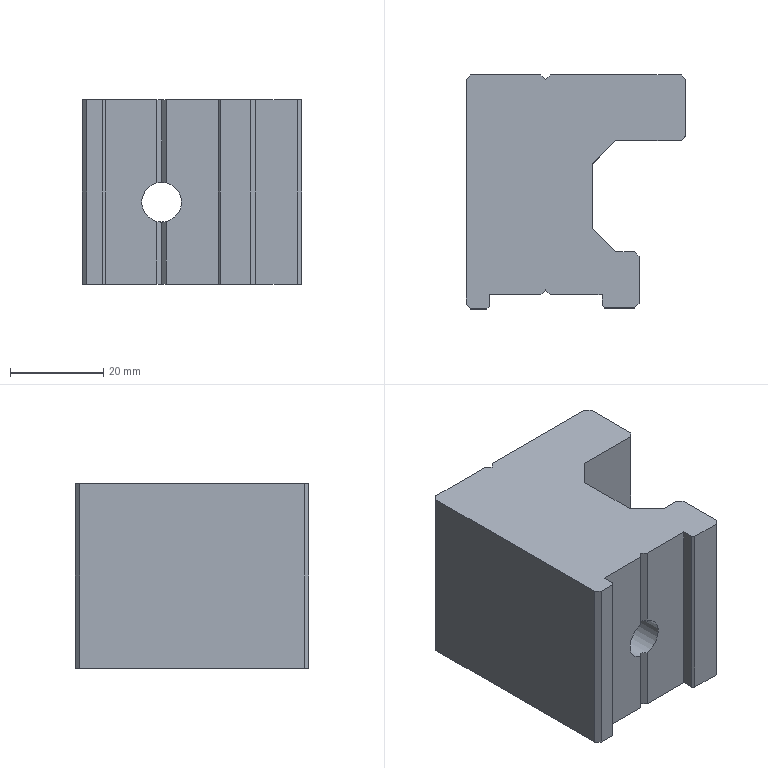Part | NX | features EXTRUDE 3, DATUM_CSYS 2, SKETCH 1 | 1 solid | 37 faces | box 47 x 50 x 39.5 mm | volume 63249 mm3 | plane 35 | cylinder 2 | commonest cylinder face diameters 8.5 x1 14 x1
STEP:
#1=CARTESIAN_POINT('',(5878.887,6899.233,-28.856));
#2=VERTEX_POINT('',#1);
#3=CARTESIAN_POINT('',(5878.887,6899.233,-15.));
#4=VERTEX_POINT('',#3);
#5=CARTESIAN_POINT('',(5879.887,6899.233,-21.928));
#6=DIRECTION('',(0.,1.,0.));
#7=DIRECTION('',(1.,0.,0.));
#8=AXIS2_PLACEMENT_3D('',#5,#6,#7);
#9=CIRCLE('',#8,7.);
#10=EDGE_CURVE('',#2,#4,#9,.T.);
#11=ORIENTED_EDGE('',*,*,#10,.F.);
#12=CARTESIAN_POINT('',(5878.887,6899.233,-39.5));
#13=VERTEX_POINT('',#12);
#14=CARTESIAN_POINT('',(5878.887,6899.233,-39.5));
#15=DIRECTION('',(0.,0.,1.));
#16=VECTOR('',#15,1000.);
#17=LINE('',#14,#16);
#18=EDGE_CURVE('',#13,#2,#17,.T.);
#19=ORIENTED_EDGE('',*,*,#18,.F.);
#20=CARTESIAN_POINT('',(5863.887,6899.233,-39.5));
#21=VERTEX_POINT('',#20);
#22=CARTESIAN_POINT('',(5863.887,6899.233,-39.5));
#23=DIRECTION('',(1.,0.,0.));
#24=VECTOR('',#23,1000.);
#25=LINE('',#22,#24);
#26=EDGE_CURVE('',#21,#13,#25,.T.);
#27=ORIENTED_EDGE('',*,*,#26,.F.);
#28=CARTESIAN_POINT('',(5863.887,6899.233,0.));
#29=VERTEX_POINT('',#28);
#30=CARTESIAN_POINT('',(5863.887,6899.233,-39.5));
#31=DIRECTION('',(0.,0.,1.));
#32=VECTOR('',#31,1000.);
#33=LINE('',#30,#32);
#34=EDGE_CURVE('',#21,#29,#33,.T.);
#35=ORIENTED_EDGE('',*,*,#34,.T.);
#36=CARTESIAN_POINT('',(5878.887,6899.233,0.));
#37=VERTEX_POINT('',#36);
#38=CARTESIAN_POINT('',(5863.887,6899.233,0.));
#39=DIRECTION('',(1.,0.,0.));
#40=VECTOR('',#39,1000.);
#41=LINE('',#38,#40);
#42=EDGE_CURVE('',#29,#37,#41,.T.);
#43=ORIENTED_EDGE('',*,*,#42,.T.);
#44=CARTESIAN_POINT('',(5878.887,6899.233,-39.5));
#45=DIRECTION('',(0.,0.,1.));
#46=VECTOR('',#45,1000.);
#47=LINE('',#44,#46);
#48=EDGE_CURVE('',#4,#37,#47,.T.);
#49=ORIENTED_EDGE('',*,*,#48,.F.);
#50=EDGE_LOOP('',(#11,#19,#27,#35,#43,#49));
#51=FACE_BOUND('',#50,.T.);
#52=CARTESIAN_POINT('',(5863.887,6899.233,-39.5));
#53=DIRECTION('',(0.,-1.,0.));
#54=DIRECTION('',(0.,0.,-1.));
#55=AXIS2_PLACEMENT_3D('',#52,#53,#54);
#56=PLANE('',#55);
#57=ADVANCED_FACE('',(#51),#56,.F.);
#58=CARTESIAN_POINT('',(5880.887,6899.233,-15.));
#59=VERTEX_POINT('',#58);
#60=CARTESIAN_POINT('',(5880.887,6899.233,-28.856));
#61=VERTEX_POINT('',#60);
#62=CARTESIAN_POINT('',(5879.887,6899.233,-21.928));
#63=DIRECTION('',(0.,1.,0.));
#64=DIRECTION('',(1.,0.,0.));
#65=AXIS2_PLACEMENT_3D('',#62,#63,#64);
#66=CIRCLE('',#65,7.);
#67=EDGE_CURVE('',#59,#61,#66,.T.);
#68=ORIENTED_EDGE('',*,*,#67,.F.);
#69=CARTESIAN_POINT('',(5880.887,6899.233,0.));
#70=VERTEX_POINT('',#69);
#71=CARTESIAN_POINT('',(5880.887,6899.233,-39.5));
#72=DIRECTION('',(0.,0.,1.));
#73=VECTOR('',#72,1000.);
#74=LINE('',#71,#73);
#75=EDGE_CURVE('',#59,#70,#74,.T.);
#76=ORIENTED_EDGE('',*,*,#75,.T.);
#77=CARTESIAN_POINT('',(5908.887,6899.233,0.));
#78=VERTEX_POINT('',#77);
#79=CARTESIAN_POINT('',(5880.887,6899.233,0.));
#80=DIRECTION('',(1.,0.,0.));
#81=VECTOR('',#80,1000.);
#82=LINE('',#79,#81);
#83=EDGE_CURVE('',#70,#78,#82,.T.);
#84=ORIENTED_EDGE('',*,*,#83,.T.);
#85=CARTESIAN_POINT('',(5908.887,6899.233,-39.5));
#86=VERTEX_POINT('',#85);
#87=CARTESIAN_POINT('',(5908.887,6899.233,-39.5));
#88=DIRECTION('',(0.,0.,1.));
#89=VECTOR('',#88,1000.);
#90=LINE('',#87,#89);
#91=EDGE_CURVE('',#86,#78,#90,.T.);
#92=ORIENTED_EDGE('',*,*,#91,.F.);
#93=CARTESIAN_POINT('',(5880.887,6899.233,-39.5));
#94=VERTEX_POINT('',#93);
#95=CARTESIAN_POINT('',(5880.887,6899.233,-39.5));
#96=DIRECTION('',(1.,0.,0.));
#97=VECTOR('',#96,1000.);
#98=LINE('',#95,#97);
#99=EDGE_CURVE('',#94,#86,#98,.T.);
#100=ORIENTED_EDGE('',*,*,#99,.F.);
#101=CARTESIAN_POINT('',(5880.887,6899.233,-39.5));
#102=DIRECTION('',(0.,0.,1.));
#103=VECTOR('',#102,1000.);
#104=LINE('',#101,#103);
#105=EDGE_CURVE('',#94,#61,#104,.T.);
#106=ORIENTED_EDGE('',*,*,#105,.T.);
#107=EDGE_LOOP('',(#68,#76,#84,#92,#100,#106));
#108=FACE_BOUND('',#107,.T.);
#109=CARTESIAN_POINT('',(5880.887,6899.233,-39.5));
#110=DIRECTION('',(0.,-1.,0.));
#111=DIRECTION('',(0.,0.,-1.));
#112=AXIS2_PLACEMENT_3D('',#109,#110,#111);
#113=PLANE('',#112);
#114=ADVANCED_FACE('',(#108),#113,.F.);
#115=CARTESIAN_POINT('',(5878.887,6852.233,-17.797));
#116=VERTEX_POINT('',#115);
#117=CARTESIAN_POINT('',(5878.887,6852.233,-26.059));
#118=VERTEX_POINT('',#117);
#119=CARTESIAN_POINT('',(5879.887,6852.233,-21.928));
#120=DIRECTION('',(0.,1.,0.));
#121=DIRECTION('',(0.,0.,1.));
#122=AXIS2_PLACEMENT_3D('',#119,#120,#121);
#123=CIRCLE('',#122,4.25);
#124=EDGE_CURVE('',#116,#118,#123,.F.);
#125=ORIENTED_EDGE('',*,*,#124,.T.);
#126=CARTESIAN_POINT('',(5879.887,6853.233,-26.178));
#127=VERTEX_POINT('',#126);
#128=CARTESIAN_POINT('',(5879.887,6853.233,-21.928));
#129=DIRECTION('',(-0.7071,0.7071,0.));
#130=DIRECTION('',(0.7071,0.7071,0.));
#131=AXIS2_PLACEMENT_3D('',#128,#129,#130);
#132=ELLIPSE('',#131,6.01,4.25);
#133=EDGE_CURVE('',#118,#127,#132,.F.);
#134=ORIENTED_EDGE('',*,*,#133,.T.);
#135=CARTESIAN_POINT('',(5880.887,6852.233,-26.059));
#136=VERTEX_POINT('',#135);
#137=CARTESIAN_POINT('',(5879.887,6853.233,-21.928));
#138=DIRECTION('',(0.7071,0.7071,0.));
#139=DIRECTION('',(-0.7071,0.7071,0.));
#140=AXIS2_PLACEMENT_3D('',#137,#138,#139);
#141=ELLIPSE('',#140,6.01,4.25);
#142=EDGE_CURVE('',#127,#136,#141,.F.);
#143=ORIENTED_EDGE('',*,*,#142,.T.);
#144=CARTESIAN_POINT('',(5880.887,6852.233,-17.797));
#145=VERTEX_POINT('',#144);
#146=CARTESIAN_POINT('',(5879.887,6852.233,-21.928));
#147=DIRECTION('',(0.,1.,0.));
#148=DIRECTION('',(0.,0.,1.));
#149=AXIS2_PLACEMENT_3D('',#146,#147,#148);
#150=CIRCLE('',#149,4.25);
#151=EDGE_CURVE('',#136,#145,#150,.F.);
#152=ORIENTED_EDGE('',*,*,#151,.T.);
#153=CARTESIAN_POINT('',(5879.887,6853.233,-17.678));
#154=VERTEX_POINT('',#153);
#155=CARTESIAN_POINT('',(5879.887,6853.233,-21.928));
#156=DIRECTION('',(0.7071,0.7071,0.));
#157=DIRECTION('',(-0.7071,0.7071,0.));
#158=AXIS2_PLACEMENT_3D('',#155,#156,#157);
#159=ELLIPSE('',#158,6.01,4.25);
#160=EDGE_CURVE('',#145,#154,#159,.F.);
#161=ORIENTED_EDGE('',*,*,#160,.T.);
#162=CARTESIAN_POINT('',(5879.887,6853.233,-21.928));
#163=DIRECTION('',(-0.7071,0.7071,0.));
#164=DIRECTION('',(0.7071,0.7071,0.));
#165=AXIS2_PLACEMENT_3D('',#162,#163,#164);
#166=ELLIPSE('',#165,6.01,4.25);
#167=EDGE_CURVE('',#154,#116,#166,.F.);
#168=ORIENTED_EDGE('',*,*,#167,.T.);
#169=EDGE_LOOP('',(#125,#134,#143,#152,#161,#168));
#170=FACE_BOUND('',#169,.T.);
#171=CARTESIAN_POINT('',(5879.887,6887.233,-17.678));
#172=VERTEX_POINT('',#171);
#173=CARTESIAN_POINT('',(5879.887,6887.233,-21.928));
#174=DIRECTION('',(0.,1.,0.));
#175=DIRECTION('',(0.,0.,1.));
#176=AXIS2_PLACEMENT_3D('',#173,#174,#175);
#177=CIRCLE('',#176,4.25);
#178=EDGE_CURVE('',#172,#172,#177,.F.);
#179=ORIENTED_EDGE('',*,*,#178,.F.);
#180=EDGE_LOOP('',(#179));
#181=FACE_BOUND('',#180,.T.);
#182=CARTESIAN_POINT('',(5879.887,-48100.767,-21.928));
#183=DIRECTION('',(0.,1.,0.));
#184=DIRECTION('',(0.,0.,1.));
#185=AXIS2_PLACEMENT_3D('',#182,#183,#184);
#186=CYLINDRICAL_SURFACE('',#185,4.25);
#187=ADVANCED_FACE('',(#170,#181),#186,.F.);
#188=ORIENTED_EDGE('',*,*,#18,.T.);
#189=CARTESIAN_POINT('',(5879.887,6898.233,-28.928));
#190=VERTEX_POINT('',#189);
#191=CARTESIAN_POINT('',(5879.887,6898.233,-21.928));
#192=DIRECTION('',(-0.7071,-0.7071,0.));
#193=DIRECTION('',(-0.7071,0.7071,0.));
#194=AXIS2_PLACEMENT_3D('',#191,#192,#193);
#195=ELLIPSE('',#194,9.899,7.);
#196=EDGE_CURVE('',#2,#190,#195,.T.);
#197=ORIENTED_EDGE('',*,*,#196,.T.);
#198=CARTESIAN_POINT('',(5879.887,6898.233,-39.5));
#199=VERTEX_POINT('',#198);
#200=CARTESIAN_POINT('',(5879.887,6898.233,-39.5));
#201=DIRECTION('',(0.,0.,1.));
#202=VECTOR('',#201,1000.);
#203=LINE('',#200,#202);
#204=EDGE_CURVE('',#199,#190,#203,.T.);
#205=ORIENTED_EDGE('',*,*,#204,.F.);
#206=CARTESIAN_POINT('',(5878.887,6899.233,-39.5));
#207=DIRECTION('',(0.7071,-0.7071,0.));
#208=VECTOR('',#207,1000.);
#209=LINE('',#206,#208);
#210=EDGE_CURVE('',#13,#199,#209,.T.);
#211=ORIENTED_EDGE('',*,*,#210,.F.);
#212=EDGE_LOOP('',(#188,#197,#205,#211));
#213=FACE_BOUND('',#212,.T.);
#214=CARTESIAN_POINT('',(5878.887,6899.233,-39.5));
#215=DIRECTION('',(-0.7071,-0.7071,0.));
#216=DIRECTION('',(0.7071,-0.7071,0.));
#217=AXIS2_PLACEMENT_3D('',#214,#215,#216);
#218=PLANE('',#217);
#219=ADVANCED_FACE('',(#213),#218,.F.);
#220=ORIENTED_EDGE('',*,*,#75,.F.);
#221=CARTESIAN_POINT('',(5879.887,6898.233,-14.928));
#222=VERTEX_POINT('',#221);
#223=CARTESIAN_POINT('',(5879.887,6898.233,-21.928));
#224=DIRECTION('',(0.7071,-0.7071,0.));
#225=DIRECTION('',(0.7071,0.7071,0.));
#226=AXIS2_PLACEMENT_3D('',#223,#224,#225);
#227=ELLIPSE('',#226,9.899,7.);
#228=EDGE_CURVE('',#59,#222,#227,.T.);
#229=ORIENTED_EDGE('',*,*,#228,.T.);
#230=CARTESIAN_POINT('',(5879.887,6898.233,0.));
#231=VERTEX_POINT('',#230);
#232=CARTESIAN_POINT('',(5879.887,6898.233,-39.5));
#233=DIRECTION('',(0.,0.,1.));
#234=VECTOR('',#233,1000.);
#235=LINE('',#232,#234);
#236=EDGE_CURVE('',#222,#231,#235,.T.);
#237=ORIENTED_EDGE('',*,*,#236,.T.);
#238=CARTESIAN_POINT('',(5879.887,6898.233,0.));
#239=DIRECTION('',(0.7071,0.7071,0.));
#240=VECTOR('',#239,1000.);
#241=LINE('',#238,#240);
#242=EDGE_CURVE('',#231,#70,#241,.T.);
#243=ORIENTED_EDGE('',*,*,#242,.T.);
#244=EDGE_LOOP('',(#220,#229,#237,#243));
#245=FACE_BOUND('',#244,.T.);
#246=CARTESIAN_POINT('',(5879.887,6898.233,-39.5));
#247=DIRECTION('',(0.7071,-0.7071,0.));
#248=DIRECTION('',(0.7071,0.7071,0.));
#249=AXIS2_PLACEMENT_3D('',#246,#247,#248);
#250=PLANE('',#249);
#251=ADVANCED_FACE('',(#245),#250,.F.);
#252=ORIENTED_EDGE('',*,*,#151,.F.);
#253=CARTESIAN_POINT('',(5880.887,6852.233,-39.5));
#254=VERTEX_POINT('',#253);
#255=CARTESIAN_POINT('',(5880.887,6852.233,-39.5));
#256=DIRECTION('',(0.,0.,1.));
#257=VECTOR('',#256,1000.);
#258=LINE('',#255,#257);
#259=EDGE_CURVE('',#254,#136,#258,.T.);
#260=ORIENTED_EDGE('',*,*,#259,.F.);
#261=CARTESIAN_POINT('',(5891.962,6852.233,-39.5));
#262=VERTEX_POINT('',#261);
#263=CARTESIAN_POINT('',(5891.962,6852.233,-39.5));
#264=DIRECTION('',(-1.,0.,0.));
#265=VECTOR('',#264,1000.);
#266=LINE('',#263,#265);
#267=EDGE_CURVE('',#262,#254,#266,.T.);
#268=ORIENTED_EDGE('',*,*,#267,.F.);
#269=CARTESIAN_POINT('',(5891.962,6852.233,0.));
#270=VERTEX_POINT('',#269);
#271=CARTESIAN_POINT('',(5891.962,6852.233,-39.5));
#272=DIRECTION('',(0.,0.,1.));
#273=VECTOR('',#272,1000.);
#274=LINE('',#271,#273);
#275=EDGE_CURVE('',#262,#270,#274,.T.);
#276=ORIENTED_EDGE('',*,*,#275,.T.);
#277=CARTESIAN_POINT('',(5880.887,6852.233,0.));
#278=VERTEX_POINT('',#277);
#279=CARTESIAN_POINT('',(5891.962,6852.233,0.));
#280=DIRECTION('',(-1.,0.,0.));
#281=VECTOR('',#280,1000.);
#282=LINE('',#279,#281);
#283=EDGE_CURVE('',#270,#278,#282,.T.);
#284=ORIENTED_EDGE('',*,*,#283,.T.);
#285=CARTESIAN_POINT('',(5880.887,6852.233,-39.5));
#286=DIRECTION('',(0.,0.,1.));
#287=VECTOR('',#286,1000.);
#288=LINE('',#285,#287);
#289=EDGE_CURVE('',#145,#278,#288,.T.);
#290=ORIENTED_EDGE('',*,*,#289,.F.);
#291=EDGE_LOOP('',(#252,#260,#268,#276,#284,#290));
#292=FACE_BOUND('',#291,.T.);
#293=CARTESIAN_POINT('',(5891.962,6852.233,-39.5));
#294=DIRECTION('',(0.,1.,0.));
#295=DIRECTION('',(0.,0.,1.));
#296=AXIS2_PLACEMENT_3D('',#293,#294,#295);
#297=PLANE('',#296);
#298=ADVANCED_FACE('',(#292),#297,.F.);
#299=ORIENTED_EDGE('',*,*,#142,.F.);
#300=CARTESIAN_POINT('',(5879.887,6853.233,-39.5));
#301=VERTEX_POINT('',#300);
#302=CARTESIAN_POINT('',(5879.887,6853.233,-39.5));
#303=DIRECTION('',(0.,0.,1.));
#304=VECTOR('',#303,1000.);
#305=LINE('',#302,#304);
#306=EDGE_CURVE('',#301,#127,#305,.T.);
#307=ORIENTED_EDGE('',*,*,#306,.F.);
#308=CARTESIAN_POINT('',(5880.887,6852.233,-39.5));
#309=DIRECTION('',(-0.7071,0.7071,0.));
#310=VECTOR('',#309,1000.);
#311=LINE('',#308,#310);
#312=EDGE_CURVE('',#254,#301,#311,.T.);
#313=ORIENTED_EDGE('',*,*,#312,.F.);
#314=ORIENTED_EDGE('',*,*,#259,.T.);
#315=EDGE_LOOP('',(#299,#307,#313,#314));
#316=FACE_BOUND('',#315,.T.);
#317=CARTESIAN_POINT('',(5880.887,6852.233,-39.5));
#318=DIRECTION('',(0.7071,0.7071,0.));
#319=DIRECTION('',(-0.7071,0.7071,0.));
#320=AXIS2_PLACEMENT_3D('',#317,#318,#319);
#321=PLANE('',#320);
#322=ADVANCED_FACE('',(#316),#321,.F.);
#323=ORIENTED_EDGE('',*,*,#160,.F.);
#324=ORIENTED_EDGE('',*,*,#289,.T.);
#325=CARTESIAN_POINT('',(5879.887,6853.233,0.));
#326=VERTEX_POINT('',#325);
#327=CARTESIAN_POINT('',(5880.887,6852.233,0.));
#328=DIRECTION('',(-0.7071,0.7071,0.));
#329=VECTOR('',#328,1000.);
#330=LINE('',#327,#329);
#331=EDGE_CURVE('',#278,#326,#330,.T.);
#332=ORIENTED_EDGE('',*,*,#331,.T.);
#333=CARTESIAN_POINT('',(5879.887,6853.233,-39.5));
#334=DIRECTION('',(0.,0.,1.));
#335=VECTOR('',#334,1000.);
#336=LINE('',#333,#335);
#337=EDGE_CURVE('',#154,#326,#336,.T.);
#338=ORIENTED_EDGE('',*,*,#337,.F.);
#339=EDGE_LOOP('',(#323,#324,#332,#338));
#340=FACE_BOUND('',#339,.T.);
#341=CARTESIAN_POINT('',(5880.887,6852.233,-39.5));
#342=DIRECTION('',(0.7071,0.7071,0.));
#343=DIRECTION('',(-0.7071,0.7071,0.));
#344=AXIS2_PLACEMENT_3D('',#341,#342,#343);
#345=PLANE('',#344);
#346=ADVANCED_FACE('',(#340),#345,.F.);
#347=ORIENTED_EDGE('',*,*,#167,.F.);
#348=ORIENTED_EDGE('',*,*,#337,.T.);
#349=CARTESIAN_POINT('',(5878.887,6852.233,0.));
#350=VERTEX_POINT('',#349);
#351=CARTESIAN_POINT('',(5879.887,6853.233,0.));
#352=DIRECTION('',(-0.7071,-0.7071,0.));
#353=VECTOR('',#352,1000.);
#354=LINE('',#351,#353);
#355=EDGE_CURVE('',#326,#350,#354,.T.);
#356=ORIENTED_EDGE('',*,*,#355,.T.);
#357=CARTESIAN_POINT('',(5878.887,6852.233,-39.5));
#358=DIRECTION('',(0.,0.,1.));
#359=VECTOR('',#358,1000.);
#360=LINE('',#357,#359);
#361=EDGE_CURVE('',#116,#350,#360,.T.);
#362=ORIENTED_EDGE('',*,*,#361,.F.);
#363=EDGE_LOOP('',(#347,#348,#356,#362));
#364=FACE_BOUND('',#363,.T.);
#365=CARTESIAN_POINT('',(5879.887,6853.233,-39.5));
#366=DIRECTION('',(-0.7071,0.7071,0.));
#367=DIRECTION('',(-0.7071,-0.7071,0.));
#368=AXIS2_PLACEMENT_3D('',#365,#366,#367);
#369=PLANE('',#368);
#370=ADVANCED_FACE('',(#364),#369,.F.);
#371=ORIENTED_EDGE('',*,*,#133,.F.);
#372=CARTESIAN_POINT('',(5878.887,6852.233,-39.5));
#373=VERTEX_POINT('',#372);
#374=CARTESIAN_POINT('',(5878.887,6852.233,-39.5));
#375=DIRECTION('',(0.,0.,1.));
#376=VECTOR('',#375,1000.);
#377=LINE('',#374,#376);
#378=EDGE_CURVE('',#373,#118,#377,.T.);
#379=ORIENTED_EDGE('',*,*,#378,.F.);
#380=CARTESIAN_POINT('',(5879.887,6853.233,-39.5));
#381=DIRECTION('',(-0.7071,-0.7071,0.));
#382=VECTOR('',#381,1000.);
#383=LINE('',#380,#382);
#384=EDGE_CURVE('',#301,#373,#383,.T.);
#385=ORIENTED_EDGE('',*,*,#384,.F.);
#386=ORIENTED_EDGE('',*,*,#306,.T.);
#387=EDGE_LOOP('',(#371,#379,#385,#386));
#388=FACE_BOUND('',#387,.T.);
#389=CARTESIAN_POINT('',(5879.887,6853.233,-39.5));
#390=DIRECTION('',(-0.7071,0.7071,0.));
#391=DIRECTION('',(-0.7071,-0.7071,0.));
#392=AXIS2_PLACEMENT_3D('',#389,#390,#391);
#393=PLANE('',#392);
#394=ADVANCED_FACE('',(#388),#393,.F.);
#395=ORIENTED_EDGE('',*,*,#124,.F.);
#396=ORIENTED_EDGE('',*,*,#361,.T.);
#397=CARTESIAN_POINT('',(5867.812,6852.233,0.));
#398=VERTEX_POINT('',#397);
#399=CARTESIAN_POINT('',(5878.887,6852.233,0.));
#400=DIRECTION('',(-1.,0.,0.));
#401=VECTOR('',#400,1000.);
#402=LINE('',#399,#401);
#403=EDGE_CURVE('',#350,#398,#402,.T.);
#404=ORIENTED_EDGE('',*,*,#403,.T.);
#405=CARTESIAN_POINT('',(5867.812,6852.233,-39.5));
#406=VERTEX_POINT('',#405);
#407=CARTESIAN_POINT('',(5867.812,6852.233,-39.5));
#408=DIRECTION('',(0.,0.,1.));
#409=VECTOR('',#408,1000.);
#410=LINE('',#407,#409);
#411=EDGE_CURVE('',#406,#398,#410,.T.);
#412=ORIENTED_EDGE('',*,*,#411,.F.);
#413=CARTESIAN_POINT('',(5878.887,6852.233,-39.5));
#414=DIRECTION('',(-1.,0.,0.));
#415=VECTOR('',#414,1000.);
#416=LINE('',#413,#415);
#417=EDGE_CURVE('',#373,#406,#416,.T.);
#418=ORIENTED_EDGE('',*,*,#417,.F.);
#419=ORIENTED_EDGE('',*,*,#378,.T.);
#420=EDGE_LOOP('',(#395,#396,#404,#412,#418,#419));
#421=FACE_BOUND('',#420,.T.);
#422=CARTESIAN_POINT('',(5878.887,6852.233,-39.5));
#423=DIRECTION('',(0.,1.,0.));
#424=DIRECTION('',(0.,0.,1.));
#425=AXIS2_PLACEMENT_3D('',#422,#423,#424);
#426=PLANE('',#425);
#427=ADVANCED_FACE('',(#421),#426,.F.);
#428=CARTESIAN_POINT('',(5862.887,6850.233,0.));
#429=VERTEX_POINT('',#428);
#430=CARTESIAN_POINT('',(5862.887,6898.233,0.));
#431=VERTEX_POINT('',#430);
#432=CARTESIAN_POINT('',(5862.887,6850.233,0.));
#433=DIRECTION('',(0.,1.,0.));
#434=VECTOR('',#433,1000.);
#435=LINE('',#432,#434);
#436=EDGE_CURVE('',#429,#431,#435,.T.);
#437=ORIENTED_EDGE('',*,*,#436,.T.);
#438=CARTESIAN_POINT('',(5862.887,6898.233,-39.5));
#439=VERTEX_POINT('',#438);
#440=CARTESIAN_POINT('',(5862.887,6898.233,-39.5));
#441=DIRECTION('',(0.,0.,1.));
#442=VECTOR('',#441,1000.);
#443=LINE('',#440,#442);
#444=EDGE_CURVE('',#439,#431,#443,.T.);
#445=ORIENTED_EDGE('',*,*,#444,.F.);
#446=CARTESIAN_POINT('',(5862.887,6850.233,-39.5));
#447=VERTEX_POINT('',#446);
#448=CARTESIAN_POINT('',(5862.887,6850.233,-39.5));
#449=DIRECTION('',(0.,1.,0.));
#450=VECTOR('',#449,1000.);
#451=LINE('',#448,#450);
#452=EDGE_CURVE('',#447,#439,#451,.T.);
#453=ORIENTED_EDGE('',*,*,#452,.F.);
#454=CARTESIAN_POINT('',(5862.887,6850.233,-39.5));
#455=DIRECTION('',(0.,0.,1.));
#456=VECTOR('',#455,1000.);
#457=LINE('',#454,#456);
#458=EDGE_CURVE('',#447,#429,#457,.T.);
#459=ORIENTED_EDGE('',*,*,#458,.T.);
#460=EDGE_LOOP('',(#437,#445,#453,#459));
#461=FACE_BOUND('',#460,.T.);
#462=CARTESIAN_POINT('',(5862.887,6850.233,-39.5));
#463=DIRECTION('',(1.,0.,0.));
#464=DIRECTION('',(0.,0.,-1.));
#465=AXIS2_PLACEMENT_3D('',#462,#463,#464);
#466=PLANE('',#465);
#467=ADVANCED_FACE('',(#461),#466,.F.);
#468=CARTESIAN_POINT('',(5862.887,6898.233,0.));
#469=DIRECTION('',(0.7071,0.7071,0.));
#470=VECTOR('',#469,1000.);
#471=LINE('',#468,#470);
#472=EDGE_CURVE('',#431,#29,#471,.T.);
#473=ORIENTED_EDGE('',*,*,#472,.T.);
#474=ORIENTED_EDGE('',*,*,#34,.F.);
#475=CARTESIAN_POINT('',(5862.887,6898.233,-39.5));
#476=DIRECTION('',(0.7071,0.7071,0.));
#477=VECTOR('',#476,1000.);
#478=LINE('',#475,#477);
#479=EDGE_CURVE('',#439,#21,#478,.T.);
#480=ORIENTED_EDGE('',*,*,#479,.F.);
#481=ORIENTED_EDGE('',*,*,#444,.T.);
#482=EDGE_LOOP('',(#473,#474,#480,#481));
#483=FACE_BOUND('',#482,.T.);
#484=CARTESIAN_POINT('',(5862.887,6898.233,-39.5));
#485=DIRECTION('',(0.7071,-0.7071,0.));
#486=DIRECTION('',(0.7071,0.7071,0.));
#487=AXIS2_PLACEMENT_3D('',#484,#485,#486);
#488=PLANE('',#487);
#489=ADVANCED_FACE('',(#483),#488,.F.);
#490=ORIENTED_EDGE('',*,*,#236,.F.);
#491=CARTESIAN_POINT('',(5879.887,6898.233,-21.928));
#492=DIRECTION('',(-0.7071,-0.7071,0.));
#493=DIRECTION('',(-0.7071,0.7071,0.));
#494=AXIS2_PLACEMENT_3D('',#491,#492,#493);
#495=ELLIPSE('',#494,9.899,7.);
#496=EDGE_CURVE('',#222,#4,#495,.T.);
#497=ORIENTED_EDGE('',*,*,#496,.T.);
#498=ORIENTED_EDGE('',*,*,#48,.T.);
#499=CARTESIAN_POINT('',(5878.887,6899.233,0.));
#500=DIRECTION('',(0.7071,-0.7071,0.));
#501=VECTOR('',#500,1000.);
#502=LINE('',#499,#501);
#503=EDGE_CURVE('',#37,#231,#502,.T.);
#504=ORIENTED_EDGE('',*,*,#503,.T.);
#505=EDGE_LOOP('',(#490,#497,#498,#504));
#506=FACE_BOUND('',#505,.T.);
#507=CARTESIAN_POINT('',(5878.887,6899.233,-39.5));
#508=DIRECTION('',(-0.7071,-0.7071,0.));
#509=DIRECTION('',(0.7071,-0.7071,0.));
#510=AXIS2_PLACEMENT_3D('',#507,#508,#509);
#511=PLANE('',#510);
#512=ADVANCED_FACE('',(#506),#511,.F.);
#513=ORIENTED_EDGE('',*,*,#204,.T.);
#514=CARTESIAN_POINT('',(5879.887,6898.233,-21.928));
#515=DIRECTION('',(0.7071,-0.7071,0.));
#516=DIRECTION('',(0.7071,0.7071,0.));
#517=AXIS2_PLACEMENT_3D('',#514,#515,#516);
#518=ELLIPSE('',#517,9.899,7.);
#519=EDGE_CURVE('',#190,#61,#518,.T.);
#520=ORIENTED_EDGE('',*,*,#519,.T.);
#521=ORIENTED_EDGE('',*,*,#105,.F.);
#522=CARTESIAN_POINT('',(5879.887,6898.233,-39.5));
#523=DIRECTION('',(0.7071,0.7071,0.));
#524=VECTOR('',#523,1000.);
#525=LINE('',#522,#524);
#526=EDGE_CURVE('',#199,#94,#525,.T.);
#527=ORIENTED_EDGE('',*,*,#526,.F.);
#528=EDGE_LOOP('',(#513,#520,#521,#527));
#529=FACE_BOUND('',#528,.T.);
#530=CARTESIAN_POINT('',(5879.887,6898.233,-39.5));
#531=DIRECTION('',(0.7071,-0.7071,0.));
#532=DIRECTION('',(0.7071,0.7071,0.));
#533=AXIS2_PLACEMENT_3D('',#530,#531,#532);
#534=PLANE('',#533);
#535=ADVANCED_FACE('',(#529),#534,.F.);
#536=CARTESIAN_POINT('',(5909.887,6898.233,0.));
#537=VERTEX_POINT('',#536);
#538=CARTESIAN_POINT('',(5908.887,6899.233,0.));
#539=DIRECTION('',(0.7071,-0.7071,0.));
#540=VECTOR('',#539,1000.);
#541=LINE('',#538,#540);
#542=EDGE_CURVE('',#78,#537,#541,.T.);
#543=ORIENTED_EDGE('',*,*,#542,.T.);
#544=CARTESIAN_POINT('',(5909.887,6898.233,-39.5));
#545=VERTEX_POINT('',#544);
#546=CARTESIAN_POINT('',(5909.887,6898.233,-39.5));
#547=DIRECTION('',(0.,0.,1.));
#548=VECTOR('',#547,1000.);
#549=LINE('',#546,#548);
#550=EDGE_CURVE('',#545,#537,#549,.T.);
#551=ORIENTED_EDGE('',*,*,#550,.F.);
#552=CARTESIAN_POINT('',(5908.887,6899.233,-39.5));
#553=DIRECTION('',(0.7071,-0.7071,0.));
#554=VECTOR('',#553,1000.);
#555=LINE('',#552,#554);
#556=EDGE_CURVE('',#86,#545,#555,.T.);
#557=ORIENTED_EDGE('',*,*,#556,.F.);
#558=ORIENTED_EDGE('',*,*,#91,.T.);
#559=EDGE_LOOP('',(#543,#551,#557,#558));
#560=FACE_BOUND('',#559,.T.);
#561=CARTESIAN_POINT('',(5908.887,6899.233,-39.5));
#562=DIRECTION('',(-0.7071,-0.7071,0.));
#563=DIRECTION('',(0.7071,-0.7071,0.));
#564=AXIS2_PLACEMENT_3D('',#561,#562,#563);
#565=PLANE('',#564);
#566=ADVANCED_FACE('',(#560),#565,.F.);
#567=CARTESIAN_POINT('',(5909.887,6886.233,0.));
#568=VERTEX_POINT('',#567);
#569=CARTESIAN_POINT('',(5909.887,6898.233,0.));
#570=DIRECTION('',(0.,-1.,0.));
#571=VECTOR('',#570,1000.);
#572=LINE('',#569,#571);
#573=EDGE_CURVE('',#537,#568,#572,.T.);
#574=ORIENTED_EDGE('',*,*,#573,.T.);
#575=CARTESIAN_POINT('',(5909.887,6886.233,-39.5));
#576=VERTEX_POINT('',#575);
#577=CARTESIAN_POINT('',(5909.887,6886.233,-39.5));
#578=DIRECTION('',(0.,0.,1.));
#579=VECTOR('',#578,1000.);
#580=LINE('',#577,#579);
#581=EDGE_CURVE('',#576,#568,#580,.T.);
#582=ORIENTED_EDGE('',*,*,#581,.F.);
#583=CARTESIAN_POINT('',(5909.887,6898.233,-39.5));
#584=DIRECTION('',(0.,-1.,0.));
#585=VECTOR('',#584,1000.);
#586=LINE('',#583,#585);
#587=EDGE_CURVE('',#545,#576,#586,.T.);
#588=ORIENTED_EDGE('',*,*,#587,.F.);
#589=ORIENTED_EDGE('',*,*,#550,.T.);
#590=EDGE_LOOP('',(#574,#582,#588,#589));
#591=FACE_BOUND('',#590,.T.);
#592=CARTESIAN_POINT('',(5909.887,6898.233,-39.5));
#593=DIRECTION('',(-1.,0.,0.));
#594=DIRECTION('',(0.,0.,1.));
#595=AXIS2_PLACEMENT_3D('',#592,#593,#594);
#596=PLANE('',#595);
#597=ADVANCED_FACE('',(#591),#596,.F.);
#598=CARTESIAN_POINT('',(5908.887,6885.233,0.));
#599=VERTEX_POINT('',#598);
#600=CARTESIAN_POINT('',(5909.887,6886.233,0.));
#601=DIRECTION('',(-0.7071,-0.7071,0.));
#602=VECTOR('',#601,1000.);
#603=LINE('',#600,#602);
#604=EDGE_CURVE('',#568,#599,#603,.T.);
#605=ORIENTED_EDGE('',*,*,#604,.T.);
#606=CARTESIAN_POINT('',(5908.887,6885.233,-39.5));
#607=VERTEX_POINT('',#606);
#608=CARTESIAN_POINT('',(5908.887,6885.233,-39.5));
#609=DIRECTION('',(0.,0.,1.));
#610=VECTOR('',#609,1000.);
#611=LINE('',#608,#610);
#612=EDGE_CURVE('',#607,#599,#611,.T.);
#613=ORIENTED_EDGE('',*,*,#612,.F.);
#614=CARTESIAN_POINT('',(5909.887,6886.233,-39.5));
#615=DIRECTION('',(-0.7071,-0.7071,0.));
#616=VECTOR('',#615,1000.);
#617=LINE('',#614,#616);
#618=EDGE_CURVE('',#576,#607,#617,.T.);
#619=ORIENTED_EDGE('',*,*,#618,.F.);
#620=ORIENTED_EDGE('',*,*,#581,.T.);
#621=EDGE_LOOP('',(#605,#613,#619,#620));
#622=FACE_BOUND('',#621,.T.);
#623=CARTESIAN_POINT('',(5909.887,6886.233,-39.5));
#624=DIRECTION('',(-0.7071,0.7071,0.));
#625=DIRECTION('',(-0.7071,-0.7071,0.));
#626=AXIS2_PLACEMENT_3D('',#623,#624,#625);
#627=PLANE('',#626);
#628=ADVANCED_FACE('',(#622),#627,.F.);
#629=CARTESIAN_POINT('',(5894.887,6885.233,0.));
#630=VERTEX_POINT('',#629);
#631=CARTESIAN_POINT('',(5908.887,6885.233,0.));
#632=DIRECTION('',(-1.,0.,0.));
#633=VECTOR('',#632,1000.);
#634=LINE('',#631,#633);
#635=EDGE_CURVE('',#599,#630,#634,.T.);
#636=ORIENTED_EDGE('',*,*,#635,.T.);
#637=CARTESIAN_POINT('',(5894.887,6885.233,-39.5));
#638=VERTEX_POINT('',#637);
#639=CARTESIAN_POINT('',(5894.887,6885.233,-39.5));
#640=DIRECTION('',(0.,0.,1.));
#641=VECTOR('',#640,1000.);
#642=LINE('',#639,#641);
#643=EDGE_CURVE('',#638,#630,#642,.T.);
#644=ORIENTED_EDGE('',*,*,#643,.F.);
#645=CARTESIAN_POINT('',(5908.887,6885.233,-39.5));
#646=DIRECTION('',(-1.,0.,0.));
#647=VECTOR('',#646,1000.);
#648=LINE('',#645,#647);
#649=EDGE_CURVE('',#607,#638,#648,.T.);
#650=ORIENTED_EDGE('',*,*,#649,.F.);
#651=ORIENTED_EDGE('',*,*,#612,.T.);
#652=EDGE_LOOP('',(#636,#644,#650,#651));
#653=FACE_BOUND('',#652,.T.);
#654=CARTESIAN_POINT('',(5908.887,6885.233,-39.5));
#655=DIRECTION('',(0.,1.,0.));
#656=DIRECTION('',(0.,0.,1.));
#657=AXIS2_PLACEMENT_3D('',#654,#655,#656);
#658=PLANE('',#657);
#659=ADVANCED_FACE('',(#653),#658,.F.);
#660=CARTESIAN_POINT('',(5889.887,6880.233,0.));
#661=VERTEX_POINT('',#660);
#662=CARTESIAN_POINT('',(5894.887,6885.233,0.));
#663=DIRECTION('',(-0.7071,-0.7071,0.));
#664=VECTOR('',#663,1000.);
#665=LINE('',#662,#664);
#666=EDGE_CURVE('',#630,#661,#665,.T.);
#667=ORIENTED_EDGE('',*,*,#666,.T.);
#668=CARTESIAN_POINT('',(5889.887,6880.233,-39.5));
#669=VERTEX_POINT('',#668);
#670=CARTESIAN_POINT('',(5889.887,6880.233,-39.5));
#671=DIRECTION('',(0.,0.,1.));
#672=VECTOR('',#671,1000.);
#673=LINE('',#670,#672);
#674=EDGE_CURVE('',#669,#661,#673,.T.);
#675=ORIENTED_EDGE('',*,*,#674,.F.);
#676=CARTESIAN_POINT('',(5894.887,6885.233,-39.5));
#677=DIRECTION('',(-0.7071,-0.7071,0.));
#678=VECTOR('',#677,1000.);
#679=LINE('',#676,#678);
#680=EDGE_CURVE('',#638,#669,#679,.T.);
#681=ORIENTED_EDGE('',*,*,#680,.F.);
#682=ORIENTED_EDGE('',*,*,#643,.T.);
#683=EDGE_LOOP('',(#667,#675,#681,#682));
#684=FACE_BOUND('',#683,.T.);
#685=CARTESIAN_POINT('',(5894.887,6885.233,-39.5));
#686=DIRECTION('',(-0.7071,0.7071,0.));
#687=DIRECTION('',(-0.7071,-0.7071,0.));
#688=AXIS2_PLACEMENT_3D('',#685,#686,#687);
#689=PLANE('',#688);
#690=ADVANCED_FACE('',(#684),#689,.F.);
#691=CARTESIAN_POINT('',(5889.887,6866.433,0.));
#692=VERTEX_POINT('',#691);
#693=CARTESIAN_POINT('',(5889.887,6880.233,0.));
#694=DIRECTION('',(0.,-1.,0.));
#695=VECTOR('',#694,1000.);
#696=LINE('',#693,#695);
#697=EDGE_CURVE('',#661,#692,#696,.T.);
#698=ORIENTED_EDGE('',*,*,#697,.T.);
#699=CARTESIAN_POINT('',(5889.887,6866.433,-39.5));
#700=VERTEX_POINT('',#699);
#701=CARTESIAN_POINT('',(5889.887,6866.433,-39.5));
#702=DIRECTION('',(0.,0.,1.));
#703=VECTOR('',#702,1000.);
#704=LINE('',#701,#703);
#705=EDGE_CURVE('',#700,#692,#704,.T.);
#706=ORIENTED_EDGE('',*,*,#705,.F.);
#707=CARTESIAN_POINT('',(5889.887,6880.233,-39.5));
#708=DIRECTION('',(0.,-1.,0.));
#709=VECTOR('',#708,1000.);
#710=LINE('',#707,#709);
#711=EDGE_CURVE('',#669,#700,#710,.T.);
#712=ORIENTED_EDGE('',*,*,#711,.F.);
#713=ORIENTED_EDGE('',*,*,#674,.T.);
#714=EDGE_LOOP('',(#698,#706,#712,#713));
#715=FACE_BOUND('',#714,.T.);
#716=CARTESIAN_POINT('',(5889.887,6880.233,-39.5));
#717=DIRECTION('',(-1.,0.,0.));
#718=DIRECTION('',(0.,0.,1.));
#719=AXIS2_PLACEMENT_3D('',#716,#717,#718);
#720=PLANE('',#719);
#721=ADVANCED_FACE('',(#715),#720,.F.);
#722=CARTESIAN_POINT('',(5894.887,6861.433,0.));
#723=VERTEX_POINT('',#722);
#724=CARTESIAN_POINT('',(5889.887,6866.433,0.));
#725=DIRECTION('',(0.7071,-0.7071,0.));
#726=VECTOR('',#725,1000.);
#727=LINE('',#724,#726);
#728=EDGE_CURVE('',#692,#723,#727,.T.);
#729=ORIENTED_EDGE('',*,*,#728,.T.);
#730=CARTESIAN_POINT('',(5894.887,6861.433,-39.5));
#731=VERTEX_POINT('',#730);
#732=CARTESIAN_POINT('',(5894.887,6861.433,-39.5));
#733=DIRECTION('',(0.,0.,1.));
#734=VECTOR('',#733,1000.);
#735=LINE('',#732,#734);
#736=EDGE_CURVE('',#731,#723,#735,.T.);
#737=ORIENTED_EDGE('',*,*,#736,.F.);
#738=CARTESIAN_POINT('',(5889.887,6866.433,-39.5));
#739=DIRECTION('',(0.7071,-0.7071,0.));
#740=VECTOR('',#739,1000.);
#741=LINE('',#738,#740);
#742=EDGE_CURVE('',#700,#731,#741,.T.);
#743=ORIENTED_EDGE('',*,*,#742,.F.);
#744=ORIENTED_EDGE('',*,*,#705,.T.);
#745=EDGE_LOOP('',(#729,#737,#743,#744));
#746=FACE_BOUND('',#745,.T.);
#747=CARTESIAN_POINT('',(5889.887,6866.433,-39.5));
#748=DIRECTION('',(-0.7071,-0.7071,0.));
#749=DIRECTION('',(0.7071,-0.7071,0.));
#750=AXIS2_PLACEMENT_3D('',#747,#748,#749);
#751=PLANE('',#750);
#752=ADVANCED_FACE('',(#746),#751,.F.);
#753=CARTESIAN_POINT('',(5898.887,6861.433,0.));
#754=VERTEX_POINT('',#753);
#755=CARTESIAN_POINT('',(5894.887,6861.433,0.));
#756=DIRECTION('',(1.,0.,0.));
#757=VECTOR('',#756,1000.);
#758=LINE('',#755,#757);
#759=EDGE_CURVE('',#723,#754,#758,.T.);
#760=ORIENTED_EDGE('',*,*,#759,.T.);
#761=CARTESIAN_POINT('',(5898.887,6861.433,-39.5));
#762=VERTEX_POINT('',#761);
#763=CARTESIAN_POINT('',(5898.887,6861.433,-39.5));
#764=DIRECTION('',(0.,0.,1.));
#765=VECTOR('',#764,1000.);
#766=LINE('',#763,#765);
#767=EDGE_CURVE('',#762,#754,#766,.T.);
#768=ORIENTED_EDGE('',*,*,#767,.F.);
#769=CARTESIAN_POINT('',(5894.887,6861.433,-39.5));
#770=DIRECTION('',(1.,0.,0.));
#771=VECTOR('',#770,1000.);
#772=LINE('',#769,#771);
#773=EDGE_CURVE('',#731,#762,#772,.T.);
#774=ORIENTED_EDGE('',*,*,#773,.F.);
#775=ORIENTED_EDGE('',*,*,#736,.T.);
#776=EDGE_LOOP('',(#760,#768,#774,#775));
#777=FACE_BOUND('',#776,.T.);
#778=CARTESIAN_POINT('',(5894.887,6861.433,-39.5));
#779=DIRECTION('',(0.,-1.,0.));
#780=DIRECTION('',(0.,0.,-1.));
#781=AXIS2_PLACEMENT_3D('',#778,#779,#780);
#782=PLANE('',#781);
#783=ADVANCED_FACE('',(#777),#782,.F.);
#784=CARTESIAN_POINT('',(5899.887,6860.433,0.));
#785=VERTEX_POINT('',#784);
#786=CARTESIAN_POINT('',(5898.887,6861.433,0.));
#787=DIRECTION('',(0.7071,-0.7071,0.));
#788=VECTOR('',#787,1000.);
#789=LINE('',#786,#788);
#790=EDGE_CURVE('',#754,#785,#789,.T.);
#791=ORIENTED_EDGE('',*,*,#790,.T.);
#792=CARTESIAN_POINT('',(5899.887,6860.433,-39.5));
#793=VERTEX_POINT('',#792);
#794=CARTESIAN_POINT('',(5899.887,6860.433,-39.5));
#795=DIRECTION('',(0.,0.,1.));
#796=VECTOR('',#795,1000.);
#797=LINE('',#794,#796);
#798=EDGE_CURVE('',#793,#785,#797,.T.);
#799=ORIENTED_EDGE('',*,*,#798,.F.);
#800=CARTESIAN_POINT('',(5898.887,6861.433,-39.5));
#801=DIRECTION('',(0.7071,-0.7071,0.));
#802=VECTOR('',#801,1000.);
#803=LINE('',#800,#802);
#804=EDGE_CURVE('',#762,#793,#803,.T.);
#805=ORIENTED_EDGE('',*,*,#804,.F.);
#806=ORIENTED_EDGE('',*,*,#767,.T.);
#807=EDGE_LOOP('',(#791,#799,#805,#806));
#808=FACE_BOUND('',#807,.T.);
#809=CARTESIAN_POINT('',(5898.887,6861.433,-39.5));
#810=DIRECTION('',(-0.7071,-0.7071,0.));
#811=DIRECTION('',(0.7071,-0.7071,0.));
#812=AXIS2_PLACEMENT_3D('',#809,#810,#811);
#813=PLANE('',#812);
#814=ADVANCED_FACE('',(#808),#813,.F.);
#815=CARTESIAN_POINT('',(5899.887,6850.433,0.));
#816=VERTEX_POINT('',#815);
#817=CARTESIAN_POINT('',(5899.887,6860.433,0.));
#818=DIRECTION('',(0.,-1.,0.));
#819=VECTOR('',#818,1000.);
#820=LINE('',#817,#819);
#821=EDGE_CURVE('',#785,#816,#820,.T.);
#822=ORIENTED_EDGE('',*,*,#821,.T.);
#823=CARTESIAN_POINT('',(5899.887,6850.433,-39.5));
#824=VERTEX_POINT('',#823);
#825=CARTESIAN_POINT('',(5899.887,6850.433,-39.5));
#826=DIRECTION('',(0.,0.,1.));
#827=VECTOR('',#826,1000.);
#828=LINE('',#825,#827);
#829=EDGE_CURVE('',#824,#816,#828,.T.);
#830=ORIENTED_EDGE('',*,*,#829,.F.);
#831=CARTESIAN_POINT('',(5899.887,6860.433,-39.5));
#832=DIRECTION('',(0.,-1.,0.));
#833=VECTOR('',#832,1000.);
#834=LINE('',#831,#833);
#835=EDGE_CURVE('',#793,#824,#834,.T.);
#836=ORIENTED_EDGE('',*,*,#835,.F.);
#837=ORIENTED_EDGE('',*,*,#798,.T.);
#838=EDGE_LOOP('',(#822,#830,#836,#837));
#839=FACE_BOUND('',#838,.T.);
#840=CARTESIAN_POINT('',(5899.887,6860.433,-39.5));
#841=DIRECTION('',(-1.,0.,0.));
#842=DIRECTION('',(0.,0.,1.));
#843=AXIS2_PLACEMENT_3D('',#840,#841,#842);
#844=PLANE('',#843);
#845=ADVANCED_FACE('',(#839),#844,.F.);
#846=CARTESIAN_POINT('',(5898.887,6849.433,0.));
#847=VERTEX_POINT('',#846);
#848=CARTESIAN_POINT('',(5899.887,6850.433,0.));
#849=DIRECTION('',(-0.7071,-0.7071,0.));
#850=VECTOR('',#849,1000.);
#851=LINE('',#848,#850);
#852=EDGE_CURVE('',#816,#847,#851,.T.);
#853=ORIENTED_EDGE('',*,*,#852,.T.);
#854=CARTESIAN_POINT('',(5898.887,6849.433,-39.5));
#855=VERTEX_POINT('',#854);
#856=CARTESIAN_POINT('',(5898.887,6849.433,-39.5));
#857=DIRECTION('',(0.,0.,1.));
#858=VECTOR('',#857,1000.);
#859=LINE('',#856,#858);
#860=EDGE_CURVE('',#855,#847,#859,.T.);
#861=ORIENTED_EDGE('',*,*,#860,.F.);
#862=CARTESIAN_POINT('',(5899.887,6850.433,-39.5));
#863=DIRECTION('',(-0.7071,-0.7071,0.));
#864=VECTOR('',#863,1000.);
#865=LINE('',#862,#864);
#866=EDGE_CURVE('',#824,#855,#865,.T.);
#867=ORIENTED_EDGE('',*,*,#866,.F.);
#868=ORIENTED_EDGE('',*,*,#829,.T.);
#869=EDGE_LOOP('',(#853,#861,#867,#868));
#870=FACE_BOUND('',#869,.T.);
#871=CARTESIAN_POINT('',(5899.887,6850.433,-39.5));
#872=DIRECTION('',(-0.7071,0.7071,0.));
#873=DIRECTION('',(-0.7071,-0.7071,0.));
#874=AXIS2_PLACEMENT_3D('',#871,#872,#873);
#875=PLANE('',#874);
#876=ADVANCED_FACE('',(#870),#875,.F.);
#877=CARTESIAN_POINT('',(5892.462,6849.433,0.));
#878=VERTEX_POINT('',#877);
#879=CARTESIAN_POINT('',(5898.887,6849.433,0.));
#880=DIRECTION('',(-1.,0.,0.));
#881=VECTOR('',#880,1000.);
#882=LINE('',#879,#881);
#883=EDGE_CURVE('',#847,#878,#882,.T.);
#884=ORIENTED_EDGE('',*,*,#883,.T.);
#885=CARTESIAN_POINT('',(5892.462,6849.433,-39.5));
#886=VERTEX_POINT('',#885);
#887=CARTESIAN_POINT('',(5892.462,6849.433,-39.5));
#888=DIRECTION('',(0.,0.,1.));
#889=VECTOR('',#888,1000.);
#890=LINE('',#887,#889);
#891=EDGE_CURVE('',#886,#878,#890,.T.);
#892=ORIENTED_EDGE('',*,*,#891,.F.);
#893=CARTESIAN_POINT('',(5898.887,6849.433,-39.5));
#894=DIRECTION('',(-1.,0.,0.));
#895=VECTOR('',#894,1000.);
#896=LINE('',#893,#895);
#897=EDGE_CURVE('',#855,#886,#896,.T.);
#898=ORIENTED_EDGE('',*,*,#897,.F.);
#899=ORIENTED_EDGE('',*,*,#860,.T.);
#900=EDGE_LOOP('',(#884,#892,#898,#899));
#901=FACE_BOUND('',#900,.T.);
#902=CARTESIAN_POINT('',(5898.887,6849.433,-39.5));
#903=DIRECTION('',(0.,1.,0.));
#904=DIRECTION('',(0.,0.,1.));
#905=AXIS2_PLACEMENT_3D('',#902,#903,#904);
#906=PLANE('',#905);
#907=ADVANCED_FACE('',(#901),#906,.F.);
#908=CARTESIAN_POINT('',(5891.962,6849.933,0.));
#909=VERTEX_POINT('',#908);
#910=CARTESIAN_POINT('',(5892.462,6849.433,0.));
#911=DIRECTION('',(-0.7071,0.7071,0.));
#912=VECTOR('',#911,1000.);
#913=LINE('',#910,#912);
#914=EDGE_CURVE('',#878,#909,#913,.T.);
#915=ORIENTED_EDGE('',*,*,#914,.T.);
#916=CARTESIAN_POINT('',(5891.962,6849.933,-39.5));
#917=VERTEX_POINT('',#916);
#918=CARTESIAN_POINT('',(5891.962,6849.933,-39.5));
#919=DIRECTION('',(0.,0.,1.));
#920=VECTOR('',#919,1000.);
#921=LINE('',#918,#920);
#922=EDGE_CURVE('',#917,#909,#921,.T.);
#923=ORIENTED_EDGE('',*,*,#922,.F.);
#924=CARTESIAN_POINT('',(5892.462,6849.433,-39.5));
#925=DIRECTION('',(-0.7071,0.7071,0.));
#926=VECTOR('',#925,1000.);
#927=LINE('',#924,#926);
#928=EDGE_CURVE('',#886,#917,#927,.T.);
#929=ORIENTED_EDGE('',*,*,#928,.F.);
#930=ORIENTED_EDGE('',*,*,#891,.T.);
#931=EDGE_LOOP('',(#915,#923,#929,#930));
#932=FACE_BOUND('',#931,.T.);
#933=CARTESIAN_POINT('',(5892.462,6849.433,-39.5));
#934=DIRECTION('',(0.7071,0.7071,0.));
#935=DIRECTION('',(-0.7071,0.7071,0.));
#936=AXIS2_PLACEMENT_3D('',#933,#934,#935);
#937=PLANE('',#936);
#938=ADVANCED_FACE('',(#932),#937,.F.);
#939=CARTESIAN_POINT('',(5891.962,6849.933,0.));
#940=DIRECTION('',(0.,1.,0.));
#941=VECTOR('',#940,1000.);
#942=LINE('',#939,#941);
#943=EDGE_CURVE('',#909,#270,#942,.T.);
#944=ORIENTED_EDGE('',*,*,#943,.T.);
#945=ORIENTED_EDGE('',*,*,#275,.F.);
#946=CARTESIAN_POINT('',(5891.962,6849.933,-39.5));
#947=DIRECTION('',(0.,1.,0.));
#948=VECTOR('',#947,1000.);
#949=LINE('',#946,#948);
#950=EDGE_CURVE('',#917,#262,#949,.T.);
#951=ORIENTED_EDGE('',*,*,#950,.F.);
#952=ORIENTED_EDGE('',*,*,#922,.T.);
#953=EDGE_LOOP('',(#944,#945,#951,#952));
#954=FACE_BOUND('',#953,.T.);
#955=CARTESIAN_POINT('',(5891.962,6849.933,-39.5));
#956=DIRECTION('',(1.,0.,0.));
#957=DIRECTION('',(0.,0.,-1.));
#958=AXIS2_PLACEMENT_3D('',#955,#956,#957);
#959=PLANE('',#958);
#960=ADVANCED_FACE('',(#954),#959,.F.);
#961=CARTESIAN_POINT('',(5867.812,6849.733,0.));
#962=VERTEX_POINT('',#961);
#963=CARTESIAN_POINT('',(5867.812,6852.233,0.));
#964=DIRECTION('',(0.,-1.,0.));
#965=VECTOR('',#964,1000.);
#966=LINE('',#963,#965);
#967=EDGE_CURVE('',#398,#962,#966,.T.);
#968=ORIENTED_EDGE('',*,*,#967,.T.);
#969=CARTESIAN_POINT('',(5867.812,6849.733,-39.5));
#970=VERTEX_POINT('',#969);
#971=CARTESIAN_POINT('',(5867.812,6849.733,-39.5));
#972=DIRECTION('',(0.,0.,1.));
#973=VECTOR('',#972,1000.);
#974=LINE('',#971,#973);
#975=EDGE_CURVE('',#970,#962,#974,.T.);
#976=ORIENTED_EDGE('',*,*,#975,.F.);
#977=CARTESIAN_POINT('',(5867.812,6852.233,-39.5));
#978=DIRECTION('',(0.,-1.,0.));
#979=VECTOR('',#978,1000.);
#980=LINE('',#977,#979);
#981=EDGE_CURVE('',#406,#970,#980,.T.);
#982=ORIENTED_EDGE('',*,*,#981,.F.);
#983=ORIENTED_EDGE('',*,*,#411,.T.);
#984=EDGE_LOOP('',(#968,#976,#982,#983));
#985=FACE_BOUND('',#984,.T.);
#986=CARTESIAN_POINT('',(5867.812,6852.233,-39.5));
#987=DIRECTION('',(-1.,0.,0.));
#988=DIRECTION('',(0.,0.,1.));
#989=AXIS2_PLACEMENT_3D('',#986,#987,#988);
#990=PLANE('',#989);
#991=ADVANCED_FACE('',(#985),#990,.F.);
#992=CARTESIAN_POINT('',(5867.312,6849.233,0.));
#993=VERTEX_POINT('',#992);
#994=CARTESIAN_POINT('',(5867.812,6849.733,0.));
#995=DIRECTION('',(-0.7071,-0.7071,0.));
#996=VECTOR('',#995,1000.);
#997=LINE('',#994,#996);
#998=EDGE_CURVE('',#962,#993,#997,.T.);
#999=ORIENTED_EDGE('',*,*,#998,.T.);
#1000=CARTESIAN_POINT('',(5867.312,6849.233,-39.5));
#1001=VERTEX_POINT('',#1000);
#1002=CARTESIAN_POINT('',(5867.312,6849.233,-39.5));
#1003=DIRECTION('',(0.,0.,1.));
#1004=VECTOR('',#1003,1000.);
#1005=LINE('',#1002,#1004);
#1006=EDGE_CURVE('',#1001,#993,#1005,.T.);
#1007=ORIENTED_EDGE('',*,*,#1006,.F.);
#1008=CARTESIAN_POINT('',(5867.812,6849.733,-39.5));
#1009=DIRECTION('',(-0.7071,-0.7071,0.));
#1010=VECTOR('',#1009,1000.);
#1011=LINE('',#1008,#1010);
#1012=EDGE_CURVE('',#970,#1001,#1011,.T.);
#1013=ORIENTED_EDGE('',*,*,#1012,.F.);
#1014=ORIENTED_EDGE('',*,*,#975,.T.);
#1015=EDGE_LOOP('',(#999,#1007,#1013,#1014));
#1016=FACE_BOUND('',#1015,.T.);
#1017=CARTESIAN_POINT('',(5867.812,6849.733,-39.5));
#1018=DIRECTION('',(-0.7071,0.7071,0.));
#1019=DIRECTION('',(-0.7071,-0.7071,0.));
#1020=AXIS2_PLACEMENT_3D('',#1017,#1018,#1019);
#1021=PLANE('',#1020);
#1022=ADVANCED_FACE('',(#1016),#1021,.F.);
#1023=CARTESIAN_POINT('',(5863.887,6849.233,0.));
#1024=VERTEX_POINT('',#1023);
#1025=CARTESIAN_POINT('',(5867.312,6849.233,0.));
#1026=DIRECTION('',(-1.,0.,0.));
#1027=VECTOR('',#1026,1000.);
#1028=LINE('',#1025,#1027);
#1029=EDGE_CURVE('',#993,#1024,#1028,.T.);
#1030=ORIENTED_EDGE('',*,*,#1029,.T.);
#1031=CARTESIAN_POINT('',(5863.887,6849.233,-39.5));
#1032=VERTEX_POINT('',#1031);
#1033=CARTESIAN_POINT('',(5863.887,6849.233,-39.5));
#1034=DIRECTION('',(0.,0.,1.));
#1035=VECTOR('',#1034,1000.);
#1036=LINE('',#1033,#1035);
#1037=EDGE_CURVE('',#1032,#1024,#1036,.T.);
#1038=ORIENTED_EDGE('',*,*,#1037,.F.);
#1039=CARTESIAN_POINT('',(5867.312,6849.233,-39.5));
#1040=DIRECTION('',(-1.,0.,0.));
#1041=VECTOR('',#1040,1000.);
#1042=LINE('',#1039,#1041);
#1043=EDGE_CURVE('',#1001,#1032,#1042,.T.);
#1044=ORIENTED_EDGE('',*,*,#1043,.F.);
#1045=ORIENTED_EDGE('',*,*,#1006,.T.);
#1046=EDGE_LOOP('',(#1030,#1038,#1044,#1045));
#1047=FACE_BOUND('',#1046,.T.);
#1048=CARTESIAN_POINT('',(5867.312,6849.233,-39.5));
#1049=DIRECTION('',(0.,1.,0.));
#1050=DIRECTION('',(0.,0.,1.));
#1051=AXIS2_PLACEMENT_3D('',#1048,#1049,#1050);
#1052=PLANE('',#1051);
#1053=ADVANCED_FACE('',(#1047),#1052,.F.);
#1054=CARTESIAN_POINT('',(5863.887,6849.233,0.));
#1055=DIRECTION('',(-0.7071,0.7071,0.));
#1056=VECTOR('',#1055,1000.);
#1057=LINE('',#1054,#1056);
#1058=EDGE_CURVE('',#1024,#429,#1057,.T.);
#1059=ORIENTED_EDGE('',*,*,#1058,.T.);
#1060=ORIENTED_EDGE('',*,*,#458,.F.);
#1061=CARTESIAN_POINT('',(5863.887,6849.233,-39.5));
#1062=DIRECTION('',(-0.7071,0.7071,0.));
#1063=VECTOR('',#1062,1000.);
#1064=LINE('',#1061,#1063);
#1065=EDGE_CURVE('',#1032,#447,#1064,.T.);
#1066=ORIENTED_EDGE('',*,*,#1065,.F.);
#1067=ORIENTED_EDGE('',*,*,#1037,.T.);
#1068=EDGE_LOOP('',(#1059,#1060,#1066,#1067));
#1069=FACE_BOUND('',#1068,.T.);
#1070=CARTESIAN_POINT('',(5863.887,6849.233,-39.5));
#1071=DIRECTION('',(0.7071,0.7071,0.));
#1072=DIRECTION('',(-0.7071,0.7071,0.));
#1073=AXIS2_PLACEMENT_3D('',#1070,#1071,#1072);
#1074=PLANE('',#1073);
#1075=ADVANCED_FACE('',(#1069),#1074,.F.);
#1076=ORIENTED_EDGE('',*,*,#452,.T.);
#1077=ORIENTED_EDGE('',*,*,#479,.T.);
#1078=ORIENTED_EDGE('',*,*,#26,.T.);
#1079=ORIENTED_EDGE('',*,*,#210,.T.);
#1080=ORIENTED_EDGE('',*,*,#526,.T.);
#1081=ORIENTED_EDGE('',*,*,#99,.T.);
#1082=ORIENTED_EDGE('',*,*,#556,.T.);
#1083=ORIENTED_EDGE('',*,*,#587,.T.);
#1084=ORIENTED_EDGE('',*,*,#618,.T.);
#1085=ORIENTED_EDGE('',*,*,#649,.T.);
#1086=ORIENTED_EDGE('',*,*,#680,.T.);
#1087=ORIENTED_EDGE('',*,*,#711,.T.);
#1088=ORIENTED_EDGE('',*,*,#742,.T.);
#1089=ORIENTED_EDGE('',*,*,#773,.T.);
#1090=ORIENTED_EDGE('',*,*,#804,.T.);
#1091=ORIENTED_EDGE('',*,*,#835,.T.);
#1092=ORIENTED_EDGE('',*,*,#866,.T.);
#1093=ORIENTED_EDGE('',*,*,#897,.T.);
#1094=ORIENTED_EDGE('',*,*,#928,.T.);
#1095=ORIENTED_EDGE('',*,*,#950,.T.);
#1096=ORIENTED_EDGE('',*,*,#267,.T.);
#1097=ORIENTED_EDGE('',*,*,#312,.T.);
#1098=ORIENTED_EDGE('',*,*,#384,.T.);
#1099=ORIENTED_EDGE('',*,*,#417,.T.);
#1100=ORIENTED_EDGE('',*,*,#981,.T.);
#1101=ORIENTED_EDGE('',*,*,#1012,.T.);
#1102=ORIENTED_EDGE('',*,*,#1043,.T.);
#1103=ORIENTED_EDGE('',*,*,#1065,.T.);
#1104=EDGE_LOOP('',(#1076,#1077,#1078,#1079,#1080,#1081,#1082,#1083,#1084,#1085,#1086,#1087,#1088,#1089,#1090,#1091,#1092,#1093,#1094,#1095,#1096,#1097,#1098,#1099,#1100,#1101,#1102,#1103));
#1105=FACE_BOUND('',#1104,.T.);
#1106=CARTESIAN_POINT('',(0.,0.,-39.5));
#1107=DIRECTION('',(0.,0.,-1.));
#1108=DIRECTION('',(0.,1.,0.));
#1109=AXIS2_PLACEMENT_3D('',#1106,#1107,#1108);
#1110=PLANE('',#1109);
#1111=ADVANCED_FACE('',(#1105),#1110,.T.);
#1112=ORIENTED_EDGE('',*,*,#436,.F.);
#1113=ORIENTED_EDGE('',*,*,#1058,.F.);
#1114=ORIENTED_EDGE('',*,*,#1029,.F.);
#1115=ORIENTED_EDGE('',*,*,#998,.F.);
#1116=ORIENTED_EDGE('',*,*,#967,.F.);
#1117=ORIENTED_EDGE('',*,*,#403,.F.);
#1118=ORIENTED_EDGE('',*,*,#355,.F.);
#1119=ORIENTED_EDGE('',*,*,#331,.F.);
#1120=ORIENTED_EDGE('',*,*,#283,.F.);
#1121=ORIENTED_EDGE('',*,*,#943,.F.);
#1122=ORIENTED_EDGE('',*,*,#914,.F.);
#1123=ORIENTED_EDGE('',*,*,#883,.F.);
#1124=ORIENTED_EDGE('',*,*,#852,.F.);
#1125=ORIENTED_EDGE('',*,*,#821,.F.);
#1126=ORIENTED_EDGE('',*,*,#790,.F.);
#1127=ORIENTED_EDGE('',*,*,#759,.F.);
#1128=ORIENTED_EDGE('',*,*,#728,.F.);
#1129=ORIENTED_EDGE('',*,*,#697,.F.);
#1130=ORIENTED_EDGE('',*,*,#666,.F.);
#1131=ORIENTED_EDGE('',*,*,#635,.F.);
#1132=ORIENTED_EDGE('',*,*,#604,.F.);
#1133=ORIENTED_EDGE('',*,*,#573,.F.);
#1134=ORIENTED_EDGE('',*,*,#542,.F.);
#1135=ORIENTED_EDGE('',*,*,#83,.F.);
#1136=ORIENTED_EDGE('',*,*,#242,.F.);
#1137=ORIENTED_EDGE('',*,*,#503,.F.);
#1138=ORIENTED_EDGE('',*,*,#42,.F.);
#1139=ORIENTED_EDGE('',*,*,#472,.F.);
#1140=EDGE_LOOP('',(#1112,#1113,#1114,#1115,#1116,#1117,#1118,#1119,#1120,#1121,#1122,#1123,#1124,#1125,#1126,#1127,#1128,#1129,#1130,#1131,#1132,#1133,#1134,#1135,#1136,#1137,#1138,#1139));
#1141=FACE_BOUND('',#1140,.T.);
#1142=CARTESIAN_POINT('',(0.,0.,0.));
#1143=DIRECTION('',(0.,0.,-1.));
#1144=DIRECTION('',(0.,1.,0.));
#1145=AXIS2_PLACEMENT_3D('',#1142,#1143,#1144);
#1146=PLANE('',#1145);
#1147=ADVANCED_FACE('',(#1141),#1146,.F.);
#1148=CARTESIAN_POINT('',(5886.887,6887.233,-21.928));
#1149=VERTEX_POINT('',#1148);
#1150=CARTESIAN_POINT('',(5879.887,6887.233,-21.928));
#1151=DIRECTION('',(0.,1.,0.));
#1152=DIRECTION('',(1.,0.,0.));
#1153=AXIS2_PLACEMENT_3D('',#1150,#1151,#1152);
#1154=CIRCLE('',#1153,7.);
#1155=EDGE_CURVE('',#1149,#1149,#1154,.F.);
#1156=ORIENTED_EDGE('',*,*,#1155,.T.);
#1157=EDGE_LOOP('',(#1156));
#1158=FACE_BOUND('',#1157,.T.);
#1159=ORIENTED_EDGE('',*,*,#67,.T.);
#1160=ORIENTED_EDGE('',*,*,#519,.F.);
#1161=ORIENTED_EDGE('',*,*,#196,.F.);
#1162=ORIENTED_EDGE('',*,*,#10,.T.);
#1163=ORIENTED_EDGE('',*,*,#496,.F.);
#1164=ORIENTED_EDGE('',*,*,#228,.F.);
#1165=EDGE_LOOP('',(#1159,#1160,#1161,#1162,#1163,#1164));
#1166=FACE_BOUND('',#1165,.T.);
#1167=CARTESIAN_POINT('',(5879.887,6887.233,-21.928));
#1168=DIRECTION('',(0.,1.,0.));
#1169=DIRECTION('',(0.,0.,1.));
#1170=AXIS2_PLACEMENT_3D('',#1167,#1168,#1169);
#1171=CYLINDRICAL_SURFACE('',#1170,7.);
#1172=ADVANCED_FACE('',(#1158,#1166),#1171,.F.);
#1173=ORIENTED_EDGE('',*,*,#1155,.F.);
#1174=EDGE_LOOP('',(#1173));
#1175=FACE_BOUND('',#1174,.T.);
#1176=ORIENTED_EDGE('',*,*,#178,.T.);
#1177=EDGE_LOOP('',(#1176));
#1178=FACE_BOUND('',#1177,.T.);
#1179=CARTESIAN_POINT('',(5879.887,6887.233,-21.928));
#1180=DIRECTION('',(0.,1.,0.));
#1181=DIRECTION('',(0.,0.,1.));
#1182=AXIS2_PLACEMENT_3D('',#1179,#1180,#1181);
#1183=PLANE('',#1182);
#1184=ADVANCED_FACE('',(#1175,#1178),#1183,.T.);
#1185=CLOSED_SHELL('',(#57,#114,#187,#219,#251,#298,#322,#346,#370,#394,#427,#467,#489,#512,#535,#566,#597,#628,#659,#690,#721,#752,#783,#814,#845,#876,#907,#938,#960,#991,#1022,#1053,#1075,#1111,#1147,#1172,#1184));
#1186=MANIFOLD_SOLID_BREP('',#1185);
#1187=(LENGTH_UNIT()NAMED_UNIT(*)SI_UNIT(.MILLI.,.METRE.));
#1188=UNCERTAINTY_MEASURE_WITH_UNIT(LENGTH_MEASURE(0.00001),#1187,'','');
#1189=(NAMED_UNIT(*)PLANE_ANGLE_UNIT()SI_UNIT($,.RADIAN.));
#1190=(NAMED_UNIT(*)SI_UNIT($,.STERADIAN.)SOLID_ANGLE_UNIT());
#1191=(GEOMETRIC_REPRESENTATION_CONTEXT(3)GLOBAL_UNCERTAINTY_ASSIGNED_CONTEXT((#1188))GLOBAL_UNIT_ASSIGNED_CONTEXT((#1187,#1189,#1190))REPRESENTATION_CONTEXT('',''));
#1192=ADVANCED_BREP_SHAPE_REPRESENTATION('',(#1186),#1191);